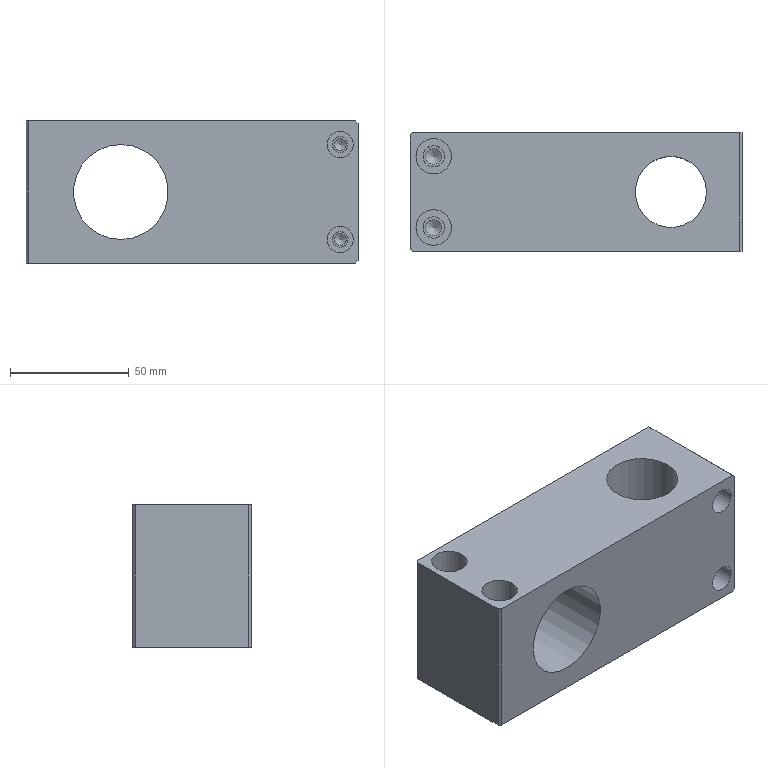CAM job | NX | 3+2 milling, drilling | part box 140 x 50 x 60 mm | stock box 145 x 55 x 65 mm
Tools:
number,name,description,diameter,corner_radius,flute_length,length,flutes
4,D4,平底铣刀-粗,4.0,0.0,25.0,75.0,2
6,D6,平底铣刀-粗,6.0,0.0,25.0,75.0,2
9,D10,平底铣刀-粗,10.0,0.0,35.0,75.0,2
18,D16,平底铣刀-粗,16.0,0.0,50.0,75.0,2
7,D6-J,平底铣刀-精,6.0,0.0,25.0,75.0,2
10,D10-J,平底铣刀-精,10.0,0.0,35.0,75.0,2
19,D16-J,平底铣刀-精,16.0,0.0,50.0,75.0,2
1,D80R0.8飞刀,圆鼻刀-粗,80.0,0.8,50.0,75.0,2
2,D6倒角刀,倒角刀,6.0,0.0,3.0,25.0,2
15,ZT5,钻头,5.0,0.0,35.0,50.0,2
16,ZT6.8,钻头,6.8,0.0,35.0,50.0,2
17,ZT12,钻头,12.0,0.0,35.0,50.0,2
Operations:
program,operation,operation_type,tool,method,geometry_group,spindle_rpm,surface_speed,feed_per_tooth,feed_cut,feed_plunge,cut_length_mm,path_length_mm,cut_time_min,machine_time_min
C,通用打点-深0.8_2,Operation,D6倒角刀,NONE,W-C,8000.0,150.796,0.0312,500.0,90.0,5.4,183.94,0.0108,0.0287
C,三段孔-G83钻孔_2,Operation,ZT6.8,NONE,W-C,3000.0,64.088,0.0333,200.0,90.0,108.586,288.188,0.5429,0.5609
C,三段孔-铣孔开粗1_2,CylinderMilling,D10,NONE,W-C,8000.0,150.796,0.075,1200.0,100.0,1001.101,1140.101,0.8343,0.8482
C,三段孔-铣孔开粗2_2,CylinderMilling,D6,NONE,W-C,8000.0,150.796,0.075,1200.0,100.0,647.786,849.786,0.5398,0.56
C,三段孔-铣孔精光1_1,CylinderMilling,D6-J,精光步距切深关,W-C,8000.0,150.796,0.0312,500.0,100.0,260.68,399.68,0.5214,0.5353
C,三段孔-铣孔精光2_1,CylinderMilling,D6-J,精光步距切深关,W-C,8000.0,150.796,0.0312,500.0,100.0,100.674,302.675,0.2013,0.2215
C,通孔-12.5-25_2,Operation,ZT12,NONE,W-C,800.0,30.159,0.1875,300.0,90.0,66.605,173.21,0.222,0.2327
C,底壁铣螺旋开粗-中_COPY,VolumeBased25DMillingOperation,D16,分层开粗-切深K-步距G,W-C,5000.0,251.327,0.3,3000.0,100.0,4443.031,4541.531,1.481,1.491
C,铣倒角_3,PlanarMilling,D6倒角刀,METHOD,W-C,8000.0,150.796,0.05,800.0,100.0,106.301,224.301,0.1329,0.1447
C,铣倒角_4,PlanarMilling,D6倒角刀,METHOD,W-C,8000.0,150.796,0.0625,1000.0,100.0,97.133,139.133,0.0971,0.1013
C,底壁铣精光侧面-中_COPY_1,VolumeBased25DMillingOperation,D16-J,侧刃精光-切深K-步距G,W-C,5000.0,251.327,0.1,1000.0,100.0,397.131,543.217,0.3971,0.4117
B,顶面_COPY,FaceMilling,D80R0.8飞刀,侧刃精光-切深K-步距G,W-B,5000.0,1256.637,0.1,1000.0,100.0,2340.0,4472.62,2.34,2.553
B,顶面_COPY_COPY,FaceMilling,D80R0.8飞刀,侧刃精光-切深K-步距G,W-B,5000.0,1256.637,0.1,1000.0,100.0,234.0,270.0,0.234,0.2376
B,C0.3平面去毛刺6X45L__COPY,SurfaceContour,D6倒角刀,爬面_倒角-切深0-步距G,W-B,8000.0,150.796,0.0938,1500.0,90.0,467.782,567.265,0.3121,0.3221
B,底壁铣倒角_COPY_1,VolumeBased25DMillingOperation,D6倒角刀,爬面_倒角-切深0-步距G,W-B,6500.0,122.519,0.1154,1500.0,100.0,68.801,109.201,0.0459,0.0499
A,顶面,FaceMilling,D80R0.8飞刀,侧刃精光-切深K-步距G,W-A,5000.0,1256.637,0.1,1000.0,100.0,234.0,270.0,0.234,0.2376
A,通用打点-深0.8,Operation,D6倒角刀,NONE,W-A,8000.0,150.796,0.0312,500.0,90.0,5.4,187.455,0.0108,0.029
A,三段孔-G83钻孔,Operation,ZT5,NONE,W-A,3000.0,47.124,0.0333,200.0,90.0,88.004,257.021,0.44,0.4569
A,通孔-12.5-25,Operation,ZT12,NONE,W-A,800.0,30.159,0.1875,300.0,90.0,59.0,158.0,0.1967,0.2066
A,外形粗_2,VolumeBased25DMillingOperation,D10,METHOD,W-A,6000.0,188.496,0.4167,5000.0,80.0,28008.27,28097.07,5.602,5.611
A,型腔铣开粗-中_COPY,CavityMilling,D10,分层开粗-切深K-步距G,W-A,6000.0,188.496,0.25,3000.0,100.0,21965.16,23789.507,7.322,7.593
A,三段孔-铣孔开粗1_1,CylinderMilling,D6,NONE,W-A,8000.0,100.531,0.075,1200.0,100.0,1670.576,1819.576,1.392,1.407
A,三段孔-铣孔开粗2_1,CylinderMilling,D4,NONE,W-A,8000.0,100.531,0.0375,600.0,100.0,678.396,880.396,1.131,1.151
A,仅选体,SurfaceContour,D6倒角刀,METHOD,W-A,8000.0,150.796,0.1875,3000.0,100.0,477.399,610.45,0.1591,0.1724
A,铣倒角_1,PlanarMilling,D6倒角刀,METHOD,W-A,8000.0,150.796,0.05,800.0,100.0,78.655,201.902,0.0983,0.1106
A,铣倒角_2,PlanarMilling,D6倒角刀,METHOD,W-A,8000.0,150.796,0.0625,1000.0,100.0,128.549,170.549,0.1285,0.1327
A,外形半精_2,VolumeBased25DMillingOperation,D10-J,METHOD,W-A,5000.0,157.08,0.1,1000.0,100.0,1305.608,1628.837,1.306,1.338
A,底壁铣倒角_COPY,VolumeBased25DMillingOperation,D6倒角刀,爬面_倒角-切深0-步距G,W-A,6500.0,122.519,0.1154,1500.0,100.0,68.801,109.201,0.0459,0.0499
A,底壁铣精光侧面-中_COPY,VolumeBased25DMillingOperation,D10-J,侧刃精光-切深K-步距G,W-A,5000.0,157.08,0.1,1000.0,100.0,617.94,739.361,0.6179,0.6301